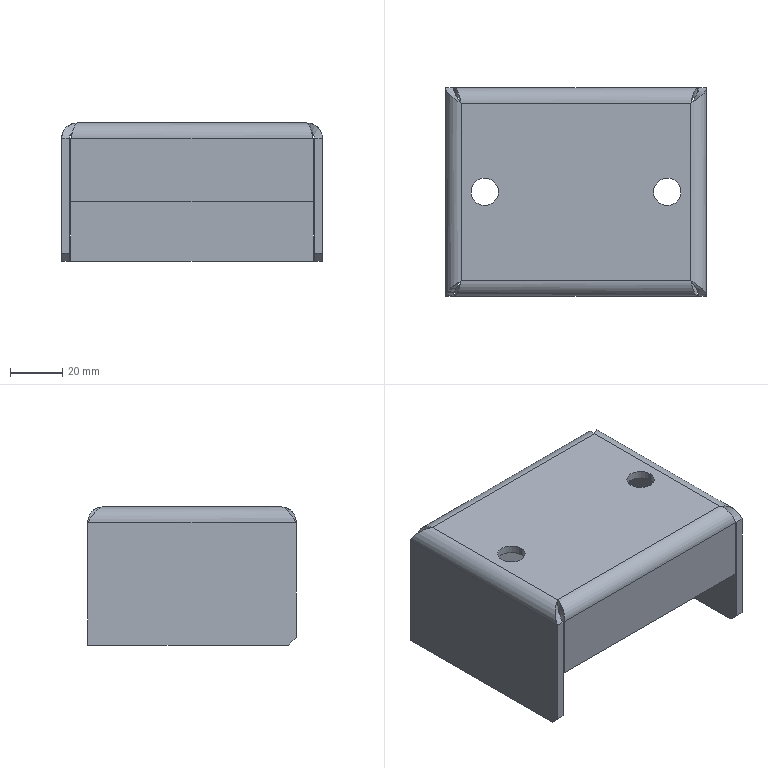Part | STEP file | SYL_0392D6J1SYL0380DJ10-1361819 | 1 solid | 44 faces | box 100 x 80 x 53 mm | volume 66751 mm3 | plane 24 | cylinder 12 | spline 8 | commonest cylinder face diameters 6 x4 10.5 x4 12 x4
STEP:
#1=CARTESIAN_POINT('',(29.75,0.,0.));
#2=VERTEX_POINT('',#1);
#3=CARTESIAN_POINT('',(29.75,0.,3.));
#4=VERTEX_POINT('',#3);
#5=CARTESIAN_POINT('',(29.75,0.,3.));
#6=DIRECTION('',(0.,0.,1.));
#7=VECTOR('',#6,1000.);
#8=LINE('',#5,#7);
#9=EDGE_CURVE('',#2,#4,#8,.T.);
#10=ORIENTED_EDGE('',*,*,#9,.F.);
#11=CARTESIAN_POINT('',(40.25,0.,0.));
#12=VERTEX_POINT('',#11);
#13=CARTESIAN_POINT('',(35.,0.,0.));
#14=DIRECTION('',(0.,0.,-1.));
#15=DIRECTION('',(-1.,0.,0.));
#16=AXIS2_PLACEMENT_3D('',#13,#14,#15);
#17=CIRCLE('',#16,5.25);
#18=EDGE_CURVE('',#2,#12,#17,.T.);
#19=ORIENTED_EDGE('',*,*,#18,.T.);
#20=CARTESIAN_POINT('',(40.25,0.,3.));
#21=VERTEX_POINT('',#20);
#22=CARTESIAN_POINT('',(40.25,0.,3.));
#23=DIRECTION('',(0.,0.,1.));
#24=VECTOR('',#23,1000.);
#25=LINE('',#22,#24);
#26=EDGE_CURVE('',#12,#21,#25,.T.);
#27=ORIENTED_EDGE('',*,*,#26,.T.);
#28=CARTESIAN_POINT('',(35.,0.,3.));
#29=DIRECTION('',(0.,0.,-1.));
#30=DIRECTION('',(-1.,0.,0.));
#31=AXIS2_PLACEMENT_3D('',#28,#29,#30);
#32=CIRCLE('',#31,5.25);
#33=EDGE_CURVE('',#4,#21,#32,.T.);
#34=ORIENTED_EDGE('',*,*,#33,.F.);
#35=EDGE_LOOP('',(#10,#19,#27,#34));
#36=FACE_OUTER_BOUND('',#35,.T.);
#37=CARTESIAN_POINT('',(35.,0.,3.));
#38=DIRECTION('',(0.,0.,1.));
#39=DIRECTION('',(1.,0.,0.));
#40=AXIS2_PLACEMENT_3D('',#37,#38,#39);
#41=CYLINDRICAL_SURFACE('',#40,5.25);
#42=ADVANCED_FACE('',(#36),#41,.F.);
#43=CARTESIAN_POINT('',(-40.25,0.,0.));
#44=VERTEX_POINT('',#43);
#45=CARTESIAN_POINT('',(-40.25,0.,3.));
#46=VERTEX_POINT('',#45);
#47=CARTESIAN_POINT('',(-40.25,0.,3.));
#48=DIRECTION('',(0.,0.,1.));
#49=VECTOR('',#48,1000.);
#50=LINE('',#47,#49);
#51=EDGE_CURVE('',#44,#46,#50,.T.);
#52=ORIENTED_EDGE('',*,*,#51,.F.);
#53=CARTESIAN_POINT('',(-29.75,0.,0.));
#54=VERTEX_POINT('',#53);
#55=CARTESIAN_POINT('',(-35.,0.,0.));
#56=DIRECTION('',(0.,0.,-1.));
#57=DIRECTION('',(-1.,0.,0.));
#58=AXIS2_PLACEMENT_3D('',#55,#56,#57);
#59=CIRCLE('',#58,5.25);
#60=EDGE_CURVE('',#44,#54,#59,.T.);
#61=ORIENTED_EDGE('',*,*,#60,.T.);
#62=CARTESIAN_POINT('',(-29.75,0.,3.));
#63=VERTEX_POINT('',#62);
#64=CARTESIAN_POINT('',(-29.75,0.,3.));
#65=DIRECTION('',(0.,0.,1.));
#66=VECTOR('',#65,1000.);
#67=LINE('',#64,#66);
#68=EDGE_CURVE('',#54,#63,#67,.T.);
#69=ORIENTED_EDGE('',*,*,#68,.T.);
#70=CARTESIAN_POINT('',(-35.,0.,3.));
#71=DIRECTION('',(0.,0.,-1.));
#72=DIRECTION('',(-1.,0.,0.));
#73=AXIS2_PLACEMENT_3D('',#70,#71,#72);
#74=CIRCLE('',#73,5.25);
#75=EDGE_CURVE('',#46,#63,#74,.T.);
#76=ORIENTED_EDGE('',*,*,#75,.F.);
#77=EDGE_LOOP('',(#52,#61,#69,#76));
#78=FACE_OUTER_BOUND('',#77,.T.);
#79=CARTESIAN_POINT('',(-35.,0.,3.));
#80=DIRECTION('',(0.,0.,1.));
#81=DIRECTION('',(1.,0.,0.));
#82=AXIS2_PLACEMENT_3D('',#79,#80,#81);
#83=CYLINDRICAL_SURFACE('',#82,5.25);
#84=ADVANCED_FACE('',(#78),#83,.F.);
#85=CARTESIAN_POINT('',(46.5,37.,-3.));
#86=VERTEX_POINT('',#85);
#87=CARTESIAN_POINT('',(46.5,40.,-3.));
#88=VERTEX_POINT('',#87);
#89=CARTESIAN_POINT('',(46.5,37.,-3.));
#90=CARTESIAN_POINT('',(46.5,40.,-3.));
#91=B_SPLINE_CURVE_WITH_KNOTS('',1,(#89,#90),.UNSPECIFIED.,.F.,.F.,(2,2),(0.,1.),.UNSPECIFIED.);
#92=EDGE_CURVE('',#86,#88,#91,.T.);
#93=ORIENTED_EDGE('',*,*,#92,.F.);
#94=CARTESIAN_POINT('',(46.5,37.,-50.));
#95=VERTEX_POINT('',#94);
#96=CARTESIAN_POINT('',(46.5,37.,3.));
#97=DIRECTION('',(0.,0.,1.));
#98=VECTOR('',#97,1000.);
#99=LINE('',#96,#98);
#100=EDGE_CURVE('',#95,#86,#99,.T.);
#101=ORIENTED_EDGE('',*,*,#100,.F.);
#102=CARTESIAN_POINT('',(46.5,40.,-50.));
#103=VERTEX_POINT('',#102);
#104=CARTESIAN_POINT('',(46.5,40.,-50.));
#105=DIRECTION('',(0.,1.,0.));
#106=VECTOR('',#105,1000.);
#107=LINE('',#104,#106);
#108=EDGE_CURVE('',#95,#103,#107,.T.);
#109=ORIENTED_EDGE('',*,*,#108,.T.);
#110=CARTESIAN_POINT('',(46.5,40.,-50.));
#111=DIRECTION('',(0.,0.,1.));
#112=VECTOR('',#111,1000.);
#113=LINE('',#110,#112);
#114=EDGE_CURVE('',#103,#88,#113,.T.);
#115=ORIENTED_EDGE('',*,*,#114,.T.);
#116=EDGE_LOOP('',(#93,#101,#109,#115));
#117=FACE_OUTER_BOUND('',#116,.T.);
#118=CARTESIAN_POINT('',(46.5,40.,-50.));
#119=DIRECTION('',(-1.,0.,0.));
#120=DIRECTION('',(0.,0.,1.));
#121=AXIS2_PLACEMENT_3D('',#118,#119,#120);
#122=PLANE('',#121);
#123=ADVANCED_FACE('',(#117),#122,.F.);
#124=ORIENTED_EDGE('',*,*,#108,.F.);
#125=CARTESIAN_POINT('',(-46.5,37.,-50.));
#126=VERTEX_POINT('',#125);
#127=CARTESIAN_POINT('',(44.,37.,-50.));
#128=DIRECTION('',(1.,0.,0.));
#129=VECTOR('',#128,1000.);
#130=LINE('',#127,#129);
#131=EDGE_CURVE('',#126,#95,#130,.T.);
#132=ORIENTED_EDGE('',*,*,#131,.F.);
#133=CARTESIAN_POINT('',(-46.5,40.,-50.));
#134=VERTEX_POINT('',#133);
#135=CARTESIAN_POINT('',(-46.5,40.,-50.));
#136=DIRECTION('',(0.,1.,0.));
#137=VECTOR('',#136,1000.);
#138=LINE('',#135,#137);
#139=EDGE_CURVE('',#126,#134,#138,.T.);
#140=ORIENTED_EDGE('',*,*,#139,.T.);
#141=CARTESIAN_POINT('',(-46.5,40.,-50.));
#142=DIRECTION('',(1.,0.,0.));
#143=VECTOR('',#142,1000.);
#144=LINE('',#141,#143);
#145=EDGE_CURVE('',#134,#103,#144,.T.);
#146=ORIENTED_EDGE('',*,*,#145,.T.);
#147=EDGE_LOOP('',(#124,#132,#140,#146));
#148=FACE_OUTER_BOUND('',#147,.T.);
#149=CARTESIAN_POINT('',(-46.5,40.,-50.));
#150=DIRECTION('',(0.,0.,1.));
#151=DIRECTION('',(1.,0.,0.));
#152=AXIS2_PLACEMENT_3D('',#149,#150,#151);
#153=PLANE('',#152);
#154=ADVANCED_FACE('',(#148),#153,.F.);
#155=ORIENTED_EDGE('',*,*,#139,.F.);
#156=CARTESIAN_POINT('',(-46.5,37.,-3.));
#157=VERTEX_POINT('',#156);
#158=CARTESIAN_POINT('',(-46.5,37.,3.));
#159=DIRECTION('',(0.,0.,1.));
#160=VECTOR('',#159,1000.);
#161=LINE('',#158,#160);
#162=EDGE_CURVE('',#126,#157,#161,.T.);
#163=ORIENTED_EDGE('',*,*,#162,.T.);
#164=CARTESIAN_POINT('',(-46.5,40.,-3.));
#165=VERTEX_POINT('',#164);
#166=CARTESIAN_POINT('',(-46.5,37.,-3.));
#167=CARTESIAN_POINT('',(-46.5,38.,-3.));
#168=CARTESIAN_POINT('',(-46.5,39.,-3.));
#169=CARTESIAN_POINT('',(-46.5,40.,-3.));
#170=B_SPLINE_CURVE_WITH_KNOTS('',3,(#166,#167,#168,#169),.UNSPECIFIED.,.F.,.F.,(4,4),(0.,1.),.UNSPECIFIED.);
#171=EDGE_CURVE('',#157,#165,#170,.T.);
#172=ORIENTED_EDGE('',*,*,#171,.T.);
#173=CARTESIAN_POINT('',(-46.5,40.,-50.));
#174=DIRECTION('',(0.,0.,1.));
#175=VECTOR('',#174,1000.);
#176=LINE('',#173,#175);
#177=EDGE_CURVE('',#134,#165,#176,.T.);
#178=ORIENTED_EDGE('',*,*,#177,.F.);
#179=EDGE_LOOP('',(#155,#163,#172,#178));
#180=FACE_OUTER_BOUND('',#179,.T.);
#181=CARTESIAN_POINT('',(-46.5,40.,-50.));
#182=DIRECTION('',(-1.,0.,0.));
#183=DIRECTION('',(0.,0.,1.));
#184=AXIS2_PLACEMENT_3D('',#181,#182,#183);
#185=PLANE('',#184);
#186=ADVANCED_FACE('',(#180),#185,.T.);
#187=ORIENTED_EDGE('',*,*,#171,.F.);
#188=CARTESIAN_POINT('',(-44.,34.,0.));
#189=VERTEX_POINT('',#188);
#190=CARTESIAN_POINT('',(-46.5,37.,-3.));
#191=CARTESIAN_POINT('',(-46.292,37.,-2.607));
#192=CARTESIAN_POINT('',(-46.083,36.922,-2.215));
#193=CARTESIAN_POINT('',(-45.667,36.621,-1.489));
#194=CARTESIAN_POINT('',(-45.458,36.399,-1.156));
#195=CARTESIAN_POINT('',(-45.042,35.844,-0.601));
#196=CARTESIAN_POINT('',(-44.833,35.511,-0.3786));
#197=CARTESIAN_POINT('',(-44.417,34.785,-0.07808));
#198=CARTESIAN_POINT('',(-44.208,34.393,0.));
#199=CARTESIAN_POINT('',(-44.,34.,0.));
#200=B_SPLINE_CURVE_WITH_KNOTS('',3,(#190,#191,#192,#193,#194,#195,#196,#197,#198,#199),.UNSPECIFIED.,.F.,.F.,(4,2,2,2,4),(0.,0.25,0.5,0.75,1.),.UNSPECIFIED.);
#201=EDGE_CURVE('',#157,#189,#200,.T.);
#202=ORIENTED_EDGE('',*,*,#201,.T.);
#203=CARTESIAN_POINT('',(-44.,34.,3.));
#204=VERTEX_POINT('',#203);
#205=CARTESIAN_POINT('',(-44.,34.,0.));
#206=CARTESIAN_POINT('',(-44.,34.,3.));
#207=B_SPLINE_CURVE_WITH_KNOTS('',1,(#205,#206),.UNSPECIFIED.,.F.,.F.,(2,2),(0.,1.),.UNSPECIFIED.);
#208=EDGE_CURVE('',#189,#204,#207,.T.);
#209=ORIENTED_EDGE('',*,*,#208,.T.);
#210=CARTESIAN_POINT('',(-46.5,40.,-3.));
#211=CARTESIAN_POINT('',(-46.292,40.,-2.215));
#212=CARTESIAN_POINT('',(-46.083,39.844,-1.43));
#213=CARTESIAN_POINT('',(-45.667,39.243,0.02171));
#214=CARTESIAN_POINT('',(-45.458,38.798,0.6873));
#215=CARTESIAN_POINT('',(-45.042,37.687,1.798));
#216=CARTESIAN_POINT('',(-44.833,37.022,2.243));
#217=CARTESIAN_POINT('',(-44.417,35.57,2.844));
#218=CARTESIAN_POINT('',(-44.208,34.785,3.));
#219=CARTESIAN_POINT('',(-44.,34.,3.));
#220=B_SPLINE_CURVE_WITH_KNOTS('',3,(#210,#211,#212,#213,#214,#215,#216,#217,#218,#219),.UNSPECIFIED.,.F.,.F.,(4,2,2,2,4),(0.,0.25,0.5,0.75,1.),.UNSPECIFIED.);
#221=EDGE_CURVE('',#165,#204,#220,.T.);
#222=ORIENTED_EDGE('',*,*,#221,.F.);
#223=EDGE_LOOP('',(#187,#202,#209,#222));
#224=FACE_OUTER_BOUND('',#223,.T.);
#225=CARTESIAN_POINT('',(-46.5,40.,-3.));
#226=CARTESIAN_POINT('',(-46.292,40.,-2.214));
#227=CARTESIAN_POINT('',(-46.083,39.844,-1.43));
#228=CARTESIAN_POINT('',(-45.667,39.243,0.02171));
#229=CARTESIAN_POINT('',(-45.458,38.798,0.6873));
#230=CARTESIAN_POINT('',(-45.042,37.687,1.798));
#231=CARTESIAN_POINT('',(-44.833,37.022,2.243));
#232=CARTESIAN_POINT('',(-44.417,35.57,2.844));
#233=CARTESIAN_POINT('',(-44.208,34.786,3.));
#234=CARTESIAN_POINT('',(-44.,34.,3.));
#235=CARTESIAN_POINT('',(-46.5,37.,-3.));
#236=CARTESIAN_POINT('',(-46.292,37.,-2.607));
#237=CARTESIAN_POINT('',(-46.083,36.922,-2.215));
#238=CARTESIAN_POINT('',(-45.667,36.621,-1.489));
#239=CARTESIAN_POINT('',(-45.458,36.399,-1.156));
#240=CARTESIAN_POINT('',(-45.042,35.844,-0.601));
#241=CARTESIAN_POINT('',(-44.833,35.511,-0.3786));
#242=CARTESIAN_POINT('',(-44.417,34.785,-0.07808));
#243=CARTESIAN_POINT('',(-44.208,34.393,0.));
#244=CARTESIAN_POINT('',(-44.,34.,0.));
#245=B_SPLINE_SURFACE_WITH_KNOTS('',1,3,((#225,#226,#227,#228,#229,#230,#231,#232,#233,#234),(#235,#236,#237,#238,#239,#240,#241,#242,#243,#244)),.UNSPECIFIED.,.F.,.F.,.F.,(2,2),(4,2,2,2,4),(0.,1.),(0.,0.25,0.5,0.75,1.),.UNSPECIFIED.);
#246=ADVANCED_FACE('',(#224),#245,.T.);
#247=ORIENTED_EDGE('',*,*,#208,.F.);
#248=CARTESIAN_POINT('',(-47.,40.,-3.));
#249=VERTEX_POINT('',#248);
#250=CARTESIAN_POINT('',(-44.,34.,0.));
#251=CARTESIAN_POINT('',(-44.393,34.5,0.));
#252=CARTESIAN_POINT('',(-44.785,35.,-0.07808));
#253=CARTESIAN_POINT('',(-45.511,36.,-0.3786));
#254=CARTESIAN_POINT('',(-45.844,36.5,-0.601));
#255=CARTESIAN_POINT('',(-46.399,37.5,-1.156));
#256=CARTESIAN_POINT('',(-46.621,38.,-1.489));
#257=CARTESIAN_POINT('',(-46.922,39.,-2.215));
#258=CARTESIAN_POINT('',(-47.,39.5,-2.607));
#259=CARTESIAN_POINT('',(-47.,40.,-3.));
#260=B_SPLINE_CURVE_WITH_KNOTS('',3,(#250,#251,#252,#253,#254,#255,#256,#257,#258,#259),.UNSPECIFIED.,.F.,.F.,(4,2,2,2,4),(0.,0.25,0.5,0.75,1.),.UNSPECIFIED.);
#261=EDGE_CURVE('',#189,#249,#260,.T.);
#262=ORIENTED_EDGE('',*,*,#261,.T.);
#263=CARTESIAN_POINT('',(-50.,40.,-3.));
#264=VERTEX_POINT('',#263);
#265=CARTESIAN_POINT('',(-47.,40.,-3.));
#266=CARTESIAN_POINT('',(-50.,40.,-3.));
#267=B_SPLINE_CURVE_WITH_KNOTS('',1,(#265,#266),.UNSPECIFIED.,.F.,.F.,(2,2),(0.,1.),.UNSPECIFIED.);
#268=EDGE_CURVE('',#249,#264,#267,.T.);
#269=ORIENTED_EDGE('',*,*,#268,.T.);
#270=CARTESIAN_POINT('',(-44.,34.,3.));
#271=CARTESIAN_POINT('',(-44.785,34.5,3.));
#272=CARTESIAN_POINT('',(-45.57,35.,2.844));
#273=CARTESIAN_POINT('',(-47.022,36.,2.243));
#274=CARTESIAN_POINT('',(-47.687,36.5,1.798));
#275=CARTESIAN_POINT('',(-48.798,37.5,0.6873));
#276=CARTESIAN_POINT('',(-49.243,38.,0.02171));
#277=CARTESIAN_POINT('',(-49.844,39.,-1.43));
#278=CARTESIAN_POINT('',(-50.,39.5,-2.215));
#279=CARTESIAN_POINT('',(-50.,40.,-3.));
#280=B_SPLINE_CURVE_WITH_KNOTS('',3,(#270,#271,#272,#273,#274,#275,#276,#277,#278,#279),.UNSPECIFIED.,.F.,.F.,(4,2,2,2,4),(0.,0.25,0.5,0.75,1.),.UNSPECIFIED.);
#281=EDGE_CURVE('',#204,#264,#280,.T.);
#282=ORIENTED_EDGE('',*,*,#281,.F.);
#283=EDGE_LOOP('',(#247,#262,#269,#282));
#284=FACE_OUTER_BOUND('',#283,.T.);
#285=CARTESIAN_POINT('',(-44.,34.,3.));
#286=CARTESIAN_POINT('',(-44.785,34.5,3.));
#287=CARTESIAN_POINT('',(-45.57,35.,2.844));
#288=CARTESIAN_POINT('',(-47.022,36.,2.243));
#289=CARTESIAN_POINT('',(-47.687,36.5,1.798));
#290=CARTESIAN_POINT('',(-48.798,37.5,0.6873));
#291=CARTESIAN_POINT('',(-49.243,38.,0.02171));
#292=CARTESIAN_POINT('',(-49.844,39.,-1.43));
#293=CARTESIAN_POINT('',(-50.,39.5,-2.215));
#294=CARTESIAN_POINT('',(-50.,40.,-3.));
#295=CARTESIAN_POINT('',(-44.,34.,0.));
#296=CARTESIAN_POINT('',(-44.393,34.5,0.));
#297=CARTESIAN_POINT('',(-44.785,35.,-0.07808));
#298=CARTESIAN_POINT('',(-45.511,36.,-0.3786));
#299=CARTESIAN_POINT('',(-45.844,36.5,-0.601));
#300=CARTESIAN_POINT('',(-46.399,37.5,-1.156));
#301=CARTESIAN_POINT('',(-46.621,38.,-1.489));
#302=CARTESIAN_POINT('',(-46.922,39.,-2.215));
#303=CARTESIAN_POINT('',(-47.,39.5,-2.607));
#304=CARTESIAN_POINT('',(-47.,40.,-3.));
#305=B_SPLINE_SURFACE_WITH_KNOTS('',1,3,((#285,#286,#287,#288,#289,#290,#291,#292,#293,#294),(#295,#296,#297,#298,#299,#300,#301,#302,#303,#304)),.UNSPECIFIED.,.F.,.F.,.F.,(2,2),(4,2,2,2,4),(0.,1.),(0.,0.25,0.5,0.75,1.),.UNSPECIFIED.);
#306=ADVANCED_FACE('',(#284),#305,.T.);
#307=ORIENTED_EDGE('',*,*,#268,.F.);
#308=CARTESIAN_POINT('',(-47.,40.,-50.));
#309=VERTEX_POINT('',#308);
#310=CARTESIAN_POINT('',(-47.,40.,3.));
#311=DIRECTION('',(0.,0.,1.));
#312=VECTOR('',#311,1000.);
#313=LINE('',#310,#312);
#314=EDGE_CURVE('',#309,#249,#313,.T.);
#315=ORIENTED_EDGE('',*,*,#314,.F.);
#316=CARTESIAN_POINT('',(-50.,40.,-50.));
#317=VERTEX_POINT('',#316);
#318=CARTESIAN_POINT('',(-50.,40.,-50.));
#319=DIRECTION('',(-1.,0.,0.));
#320=VECTOR('',#319,1000.);
#321=LINE('',#318,#320);
#322=EDGE_CURVE('',#309,#317,#321,.T.);
#323=ORIENTED_EDGE('',*,*,#322,.T.);
#324=CARTESIAN_POINT('',(-50.,40.,-50.));
#325=DIRECTION('',(0.,0.,1.));
#326=VECTOR('',#325,1000.);
#327=LINE('',#324,#326);
#328=EDGE_CURVE('',#317,#264,#327,.T.);
#329=ORIENTED_EDGE('',*,*,#328,.T.);
#330=EDGE_LOOP('',(#307,#315,#323,#329));
#331=FACE_OUTER_BOUND('',#330,.T.);
#332=CARTESIAN_POINT('',(-50.,40.,-50.));
#333=DIRECTION('',(0.,-1.,0.));
#334=DIRECTION('',(0.,0.,1.));
#335=AXIS2_PLACEMENT_3D('',#332,#333,#334);
#336=PLANE('',#335);
#337=ADVANCED_FACE('',(#331),#336,.F.);
#338=ORIENTED_EDGE('',*,*,#322,.F.);
#339=CARTESIAN_POINT('',(-47.,-37.,-50.));
#340=VERTEX_POINT('',#339);
#341=CARTESIAN_POINT('',(-47.,40.,-50.));
#342=DIRECTION('',(0.,1.,0.));
#343=VECTOR('',#342,1000.);
#344=LINE('',#341,#343);
#345=EDGE_CURVE('',#340,#309,#344,.T.);
#346=ORIENTED_EDGE('',*,*,#345,.F.);
#347=CARTESIAN_POINT('',(-50.,-37.,-50.));
#348=VERTEX_POINT('',#347);
#349=CARTESIAN_POINT('',(-50.,-37.,-50.));
#350=DIRECTION('',(-1.,0.,0.));
#351=VECTOR('',#350,1000.);
#352=LINE('',#349,#351);
#353=EDGE_CURVE('',#340,#348,#352,.T.);
#354=ORIENTED_EDGE('',*,*,#353,.T.);
#355=CARTESIAN_POINT('',(-50.,-37.,-50.));
#356=DIRECTION('',(0.,1.,0.));
#357=VECTOR('',#356,1000.);
#358=LINE('',#355,#357);
#359=EDGE_CURVE('',#348,#317,#358,.T.);
#360=ORIENTED_EDGE('',*,*,#359,.T.);
#361=EDGE_LOOP('',(#338,#346,#354,#360));
#362=FACE_OUTER_BOUND('',#361,.T.);
#363=CARTESIAN_POINT('',(-50.,-37.,-50.));
#364=DIRECTION('',(0.,0.,1.));
#365=DIRECTION('',(0.,1.,0.));
#366=AXIS2_PLACEMENT_3D('',#363,#364,#365);
#367=PLANE('',#366);
#368=ADVANCED_FACE('',(#362),#367,.F.);
#369=ORIENTED_EDGE('',*,*,#353,.F.);
#370=CARTESIAN_POINT('',(-47.,-40.,-47.));
#371=VERTEX_POINT('',#370);
#372=CARTESIAN_POINT('',(-47.,-37.,-50.));
#373=DIRECTION('',(0.,-0.7071,0.7071));
#374=VECTOR('',#373,1000.);
#375=LINE('',#372,#374);
#376=EDGE_CURVE('',#340,#371,#375,.T.);
#377=ORIENTED_EDGE('',*,*,#376,.T.);
#378=CARTESIAN_POINT('',(-50.,-40.,-47.));
#379=VERTEX_POINT('',#378);
#380=CARTESIAN_POINT('',(-50.,-40.,-47.));
#381=DIRECTION('',(-1.,0.,0.));
#382=VECTOR('',#381,1000.);
#383=LINE('',#380,#382);
#384=EDGE_CURVE('',#371,#379,#383,.T.);
#385=ORIENTED_EDGE('',*,*,#384,.T.);
#386=CARTESIAN_POINT('',(-50.,-37.,-50.));
#387=DIRECTION('',(0.,-0.7071,0.7071));
#388=VECTOR('',#387,1000.);
#389=LINE('',#386,#388);
#390=EDGE_CURVE('',#348,#379,#389,.T.);
#391=ORIENTED_EDGE('',*,*,#390,.F.);
#392=EDGE_LOOP('',(#369,#377,#385,#391));
#393=FACE_OUTER_BOUND('',#392,.T.);
#394=CARTESIAN_POINT('',(-50.,-37.,-50.));
#395=DIRECTION('',(0.,-0.7071,-0.7071));
#396=DIRECTION('',(0.,-0.7071,0.7071));
#397=AXIS2_PLACEMENT_3D('',#394,#395,#396);
#398=PLANE('',#397);
#399=ADVANCED_FACE('',(#393),#398,.T.);
#400=ORIENTED_EDGE('',*,*,#384,.F.);
#401=CARTESIAN_POINT('',(-47.,-40.,-3.));
#402=VERTEX_POINT('',#401);
#403=CARTESIAN_POINT('',(-47.,-40.,3.));
#404=DIRECTION('',(0.,0.,1.));
#405=VECTOR('',#404,1000.);
#406=LINE('',#403,#405);
#407=EDGE_CURVE('',#371,#402,#406,.T.);
#408=ORIENTED_EDGE('',*,*,#407,.T.);
#409=CARTESIAN_POINT('',(-50.,-40.,-3.));
#410=VERTEX_POINT('',#409);
#411=CARTESIAN_POINT('',(-47.,-40.,-3.));
#412=CARTESIAN_POINT('',(-48.,-40.,-3.));
#413=CARTESIAN_POINT('',(-49.,-40.,-3.));
#414=CARTESIAN_POINT('',(-50.,-40.,-3.));
#415=B_SPLINE_CURVE_WITH_KNOTS('',3,(#411,#412,#413,#414),.UNSPECIFIED.,.F.,.F.,(4,4),(0.,1.),.UNSPECIFIED.);
#416=EDGE_CURVE('',#402,#410,#415,.T.);
#417=ORIENTED_EDGE('',*,*,#416,.T.);
#418=CARTESIAN_POINT('',(-50.,-40.,-47.));
#419=DIRECTION('',(0.,0.,1.));
#420=VECTOR('',#419,1000.);
#421=LINE('',#418,#420);
#422=EDGE_CURVE('',#379,#410,#421,.T.);
#423=ORIENTED_EDGE('',*,*,#422,.F.);
#424=EDGE_LOOP('',(#400,#408,#417,#423));
#425=FACE_OUTER_BOUND('',#424,.T.);
#426=CARTESIAN_POINT('',(-50.,-40.,-47.));
#427=DIRECTION('',(0.,-1.,0.));
#428=DIRECTION('',(0.,0.,1.));
#429=AXIS2_PLACEMENT_3D('',#426,#427,#428);
#430=PLANE('',#429);
#431=ADVANCED_FACE('',(#425),#430,.T.);
#432=ORIENTED_EDGE('',*,*,#416,.F.);
#433=CARTESIAN_POINT('',(-44.,-34.,0.));
#434=VERTEX_POINT('',#433);
#435=CARTESIAN_POINT('',(-47.,-40.,-3.));
#436=CARTESIAN_POINT('',(-47.,-39.5,-2.607));
#437=CARTESIAN_POINT('',(-46.922,-39.,-2.215));
#438=CARTESIAN_POINT('',(-46.621,-38.,-1.489));
#439=CARTESIAN_POINT('',(-46.399,-37.5,-1.156));
#440=CARTESIAN_POINT('',(-45.844,-36.5,-0.601));
#441=CARTESIAN_POINT('',(-45.511,-36.,-0.3786));
#442=CARTESIAN_POINT('',(-44.785,-35.,-0.07808));
#443=CARTESIAN_POINT('',(-44.393,-34.5,0.));
#444=CARTESIAN_POINT('',(-44.,-34.,0.));
#445=B_SPLINE_CURVE_WITH_KNOTS('',3,(#435,#436,#437,#438,#439,#440,#441,#442,#443,#444),.UNSPECIFIED.,.F.,.F.,(4,2,2,2,4),(0.,0.25,0.5,0.75,1.),.UNSPECIFIED.);
#446=EDGE_CURVE('',#402,#434,#445,.T.);
#447=ORIENTED_EDGE('',*,*,#446,.T.);
#448=CARTESIAN_POINT('',(-44.,-34.,3.));
#449=VERTEX_POINT('',#448);
#450=CARTESIAN_POINT('',(-44.,-34.,0.));
#451=CARTESIAN_POINT('',(-44.,-34.,3.));
#452=B_SPLINE_CURVE_WITH_KNOTS('',1,(#450,#451),.UNSPECIFIED.,.F.,.F.,(2,2),(0.,1.),.UNSPECIFIED.);
#453=EDGE_CURVE('',#434,#449,#452,.T.);
#454=ORIENTED_EDGE('',*,*,#453,.T.);
#455=CARTESIAN_POINT('',(-50.,-40.,-3.));
#456=CARTESIAN_POINT('',(-50.,-39.5,-2.215));
#457=CARTESIAN_POINT('',(-49.844,-39.,-1.43));
#458=CARTESIAN_POINT('',(-49.243,-38.,0.02171));
#459=CARTESIAN_POINT('',(-48.798,-37.5,0.6873));
#460=CARTESIAN_POINT('',(-47.687,-36.5,1.798));
#461=CARTESIAN_POINT('',(-47.022,-36.,2.243));
#462=CARTESIAN_POINT('',(-45.57,-35.,2.844));
#463=CARTESIAN_POINT('',(-44.785,-34.5,3.));
#464=CARTESIAN_POINT('',(-44.,-34.,3.));
#465=B_SPLINE_CURVE_WITH_KNOTS('',3,(#455,#456,#457,#458,#459,#460,#461,#462,#463,#464),.UNSPECIFIED.,.F.,.F.,(4,2,2,2,4),(0.,0.25,0.5,0.75,1.),.UNSPECIFIED.);
#466=EDGE_CURVE('',#410,#449,#465,.T.);
#467=ORIENTED_EDGE('',*,*,#466,.F.);
#468=EDGE_LOOP('',(#432,#447,#454,#467));
#469=FACE_OUTER_BOUND('',#468,.T.);
#470=CARTESIAN_POINT('',(-50.,-40.,-3.));
#471=CARTESIAN_POINT('',(-50.,-39.5,-2.215));
#472=CARTESIAN_POINT('',(-49.844,-39.,-1.43));
#473=CARTESIAN_POINT('',(-49.243,-38.,0.02171));
#474=CARTESIAN_POINT('',(-48.798,-37.5,0.6873));
#475=CARTESIAN_POINT('',(-47.687,-36.5,1.798));
#476=CARTESIAN_POINT('',(-47.022,-36.,2.243));
#477=CARTESIAN_POINT('',(-45.57,-35.,2.844));
#478=CARTESIAN_POINT('',(-44.785,-34.5,3.));
#479=CARTESIAN_POINT('',(-44.,-34.,3.));
#480=CARTESIAN_POINT('',(-47.,-40.,-3.));
#481=CARTESIAN_POINT('',(-47.,-39.5,-2.607));
#482=CARTESIAN_POINT('',(-46.922,-39.,-2.215));
#483=CARTESIAN_POINT('',(-46.621,-38.,-1.489));
#484=CARTESIAN_POINT('',(-46.399,-37.5,-1.156));
#485=CARTESIAN_POINT('',(-45.844,-36.5,-0.601));
#486=CARTESIAN_POINT('',(-45.511,-36.,-0.3786));
#487=CARTESIAN_POINT('',(-44.785,-35.,-0.07808));
#488=CARTESIAN_POINT('',(-44.393,-34.5,0.));
#489=CARTESIAN_POINT('',(-44.,-34.,0.));
#490=B_SPLINE_SURFACE_WITH_KNOTS('',1,3,((#470,#471,#472,#473,#474,#475,#476,#477,#478,#479),(#480,#481,#482,#483,#484,#485,#486,#487,#488,#489)),.UNSPECIFIED.,.F.,.F.,.F.,(2,2),(4,2,2,2,4),(0.,1.),(0.,0.25,0.5,0.75,1.),.UNSPECIFIED.);
#491=ADVANCED_FACE('',(#469),#490,.T.);
#492=ORIENTED_EDGE('',*,*,#453,.F.);
#493=CARTESIAN_POINT('',(-46.5,-37.,-3.));
#494=VERTEX_POINT('',#493);
#495=CARTESIAN_POINT('',(-44.,-34.,0.));
#496=CARTESIAN_POINT('',(-44.208,-34.393,0.));
#497=CARTESIAN_POINT('',(-44.417,-34.785,-0.07808));
#498=CARTESIAN_POINT('',(-44.833,-35.511,-0.3786));
#499=CARTESIAN_POINT('',(-45.042,-35.844,-0.601));
#500=CARTESIAN_POINT('',(-45.458,-36.399,-1.156));
#501=CARTESIAN_POINT('',(-45.667,-36.621,-1.489));
#502=CARTESIAN_POINT('',(-46.083,-36.922,-2.215));
#503=CARTESIAN_POINT('',(-46.292,-37.,-2.607));
#504=CARTESIAN_POINT('',(-46.5,-37.,-3.));
#505=B_SPLINE_CURVE_WITH_KNOTS('',3,(#495,#496,#497,#498,#499,#500,#501,#502,#503,#504),.UNSPECIFIED.,.F.,.F.,(4,2,2,2,4),(0.,0.25,0.5,0.75,1.),.UNSPECIFIED.);
#506=EDGE_CURVE('',#434,#494,#505,.T.);
#507=ORIENTED_EDGE('',*,*,#506,.T.);
#508=CARTESIAN_POINT('',(-46.5,-40.,-3.));
#509=VERTEX_POINT('',#508);
#510=CARTESIAN_POINT('',(-46.5,-37.,-3.));
#511=CARTESIAN_POINT('',(-46.5,-40.,-3.));
#512=B_SPLINE_CURVE_WITH_KNOTS('',1,(#510,#511),.UNSPECIFIED.,.F.,.F.,(2,2),(0.,1.),.UNSPECIFIED.);
#513=EDGE_CURVE('',#494,#509,#512,.T.);
#514=ORIENTED_EDGE('',*,*,#513,.T.);
#515=CARTESIAN_POINT('',(-44.,-34.,3.));
#516=CARTESIAN_POINT('',(-44.208,-34.785,3.));
#517=CARTESIAN_POINT('',(-44.417,-35.57,2.844));
#518=CARTESIAN_POINT('',(-44.833,-37.022,2.243));
#519=CARTESIAN_POINT('',(-45.042,-37.687,1.798));
#520=CARTESIAN_POINT('',(-45.458,-38.798,0.6873));
#521=CARTESIAN_POINT('',(-45.667,-39.243,0.02171));
#522=CARTESIAN_POINT('',(-46.083,-39.844,-1.43));
#523=CARTESIAN_POINT('',(-46.292,-40.,-2.215));
#524=CARTESIAN_POINT('',(-46.5,-40.,-3.));
#525=B_SPLINE_CURVE_WITH_KNOTS('',3,(#515,#516,#517,#518,#519,#520,#521,#522,#523,#524),.UNSPECIFIED.,.F.,.F.,(4,2,2,2,4),(0.,0.25,0.5,0.75,1.),.UNSPECIFIED.);
#526=EDGE_CURVE('',#449,#509,#525,.T.);
#527=ORIENTED_EDGE('',*,*,#526,.F.);
#528=EDGE_LOOP('',(#492,#507,#514,#527));
#529=FACE_OUTER_BOUND('',#528,.T.);
#530=CARTESIAN_POINT('',(-44.,-34.,3.));
#531=CARTESIAN_POINT('',(-44.208,-34.786,3.));
#532=CARTESIAN_POINT('',(-44.417,-35.57,2.844));
#533=CARTESIAN_POINT('',(-44.833,-37.022,2.243));
#534=CARTESIAN_POINT('',(-45.042,-37.687,1.798));
#535=CARTESIAN_POINT('',(-45.458,-38.798,0.6873));
#536=CARTESIAN_POINT('',(-45.667,-39.243,0.02171));
#537=CARTESIAN_POINT('',(-46.083,-39.844,-1.43));
#538=CARTESIAN_POINT('',(-46.292,-40.,-2.214));
#539=CARTESIAN_POINT('',(-46.5,-40.,-3.));
#540=CARTESIAN_POINT('',(-44.,-34.,0.));
#541=CARTESIAN_POINT('',(-44.208,-34.393,0.));
#542=CARTESIAN_POINT('',(-44.417,-34.785,-0.07808));
#543=CARTESIAN_POINT('',(-44.833,-35.511,-0.3786));
#544=CARTESIAN_POINT('',(-45.042,-35.844,-0.601));
#545=CARTESIAN_POINT('',(-45.458,-36.399,-1.156));
#546=CARTESIAN_POINT('',(-45.667,-36.621,-1.489));
#547=CARTESIAN_POINT('',(-46.083,-36.922,-2.215));
#548=CARTESIAN_POINT('',(-46.292,-37.,-2.607));
#549=CARTESIAN_POINT('',(-46.5,-37.,-3.));
#550=B_SPLINE_SURFACE_WITH_KNOTS('',1,3,((#530,#531,#532,#533,#534,#535,#536,#537,#538,#539),(#540,#541,#542,#543,#544,#545,#546,#547,#548,#549)),.UNSPECIFIED.,.F.,.F.,.F.,(2,2),(4,2,2,2,4),(0.,1.),(0.,0.25,0.5,0.75,1.),.UNSPECIFIED.);
#551=ADVANCED_FACE('',(#529),#550,.T.);
#552=ORIENTED_EDGE('',*,*,#513,.F.);
#553=CARTESIAN_POINT('',(-46.5,-37.,-27.));
#554=VERTEX_POINT('',#553);
#555=CARTESIAN_POINT('',(-46.5,-37.,3.));
#556=DIRECTION('',(0.,0.,1.));
#557=VECTOR('',#556,1000.);
#558=LINE('',#555,#557);
#559=EDGE_CURVE('',#554,#494,#558,.T.);
#560=ORIENTED_EDGE('',*,*,#559,.F.);
#561=CARTESIAN_POINT('',(-46.5,-40.,-27.));
#562=VERTEX_POINT('',#561);
#563=CARTESIAN_POINT('',(-46.5,-40.,-27.));
#564=DIRECTION('',(0.,-1.,0.));
#565=VECTOR('',#564,1000.);
#566=LINE('',#563,#565);
#567=EDGE_CURVE('',#554,#562,#566,.T.);
#568=ORIENTED_EDGE('',*,*,#567,.T.);
#569=CARTESIAN_POINT('',(-46.5,-40.,-27.));
#570=DIRECTION('',(0.,0.,1.));
#571=VECTOR('',#570,1000.);
#572=LINE('',#569,#571);
#573=EDGE_CURVE('',#562,#509,#572,.T.);
#574=ORIENTED_EDGE('',*,*,#573,.T.);
#575=EDGE_LOOP('',(#552,#560,#568,#574));
#576=FACE_OUTER_BOUND('',#575,.T.);
#577=CARTESIAN_POINT('',(-46.5,-40.,-27.));
#578=DIRECTION('',(1.,0.,0.));
#579=DIRECTION('',(0.,0.,1.));
#580=AXIS2_PLACEMENT_3D('',#577,#578,#579);
#581=PLANE('',#580);
#582=ADVANCED_FACE('',(#576),#581,.F.);
#583=ORIENTED_EDGE('',*,*,#567,.F.);
#584=CARTESIAN_POINT('',(46.5,-37.,-27.));
#585=VERTEX_POINT('',#584);
#586=CARTESIAN_POINT('',(-44.,-37.,-27.));
#587=DIRECTION('',(-1.,0.,0.));
#588=VECTOR('',#587,1000.);
#589=LINE('',#586,#588);
#590=EDGE_CURVE('',#585,#554,#589,.T.);
#591=ORIENTED_EDGE('',*,*,#590,.F.);
#592=CARTESIAN_POINT('',(46.5,-40.,-27.));
#593=VERTEX_POINT('',#592);
#594=CARTESIAN_POINT('',(46.5,-40.,-27.));
#595=DIRECTION('',(0.,-1.,0.));
#596=VECTOR('',#595,1000.);
#597=LINE('',#594,#596);
#598=EDGE_CURVE('',#585,#593,#597,.T.);
#599=ORIENTED_EDGE('',*,*,#598,.T.);
#600=CARTESIAN_POINT('',(46.5,-40.,-27.));
#601=DIRECTION('',(-1.,0.,0.));
#602=VECTOR('',#601,1000.);
#603=LINE('',#600,#602);
#604=EDGE_CURVE('',#593,#562,#603,.T.);
#605=ORIENTED_EDGE('',*,*,#604,.T.);
#606=EDGE_LOOP('',(#583,#591,#599,#605));
#607=FACE_OUTER_BOUND('',#606,.T.);
#608=CARTESIAN_POINT('',(46.5,-40.,-27.));
#609=DIRECTION('',(0.,0.,1.));
#610=DIRECTION('',(-1.,0.,0.));
#611=AXIS2_PLACEMENT_3D('',#608,#609,#610);
#612=PLANE('',#611);
#613=ADVANCED_FACE('',(#607),#612,.F.);
#614=ORIENTED_EDGE('',*,*,#598,.F.);
#615=CARTESIAN_POINT('',(46.5,-37.,-3.));
#616=VERTEX_POINT('',#615);
#617=CARTESIAN_POINT('',(46.5,-37.,3.));
#618=DIRECTION('',(0.,0.,1.));
#619=VECTOR('',#618,1000.);
#620=LINE('',#617,#619);
#621=EDGE_CURVE('',#585,#616,#620,.T.);
#622=ORIENTED_EDGE('',*,*,#621,.T.);
#623=CARTESIAN_POINT('',(46.5,-40.,-3.));
#624=VERTEX_POINT('',#623);
#625=CARTESIAN_POINT('',(46.5,-37.,-3.));
#626=CARTESIAN_POINT('',(46.5,-38.,-3.));
#627=CARTESIAN_POINT('',(46.5,-39.,-3.));
#628=CARTESIAN_POINT('',(46.5,-40.,-3.));
#629=B_SPLINE_CURVE_WITH_KNOTS('',3,(#625,#626,#627,#628),.UNSPECIFIED.,.F.,.F.,(4,4),(0.,1.),.UNSPECIFIED.);
#630=EDGE_CURVE('',#616,#624,#629,.T.);
#631=ORIENTED_EDGE('',*,*,#630,.T.);
#632=CARTESIAN_POINT('',(46.5,-40.,-27.));
#633=DIRECTION('',(0.,0.,1.));
#634=VECTOR('',#633,1000.);
#635=LINE('',#632,#634);
#636=EDGE_CURVE('',#593,#624,#635,.T.);
#637=ORIENTED_EDGE('',*,*,#636,.F.);
#638=EDGE_LOOP('',(#614,#622,#631,#637));
#639=FACE_OUTER_BOUND('',#638,.T.);
#640=CARTESIAN_POINT('',(46.5,-40.,-27.));
#641=DIRECTION('',(1.,0.,0.));
#642=DIRECTION('',(0.,0.,1.));
#643=AXIS2_PLACEMENT_3D('',#640,#641,#642);
#644=PLANE('',#643);
#645=ADVANCED_FACE('',(#639),#644,.T.);
#646=ORIENTED_EDGE('',*,*,#630,.F.);
#647=CARTESIAN_POINT('',(44.,-34.,0.));
#648=VERTEX_POINT('',#647);
#649=CARTESIAN_POINT('',(46.5,-37.,-3.));
#650=CARTESIAN_POINT('',(46.292,-37.,-2.607));
#651=CARTESIAN_POINT('',(46.083,-36.922,-2.215));
#652=CARTESIAN_POINT('',(45.667,-36.621,-1.489));
#653=CARTESIAN_POINT('',(45.458,-36.399,-1.156));
#654=CARTESIAN_POINT('',(45.042,-35.844,-0.601));
#655=CARTESIAN_POINT('',(44.833,-35.511,-0.3786));
#656=CARTESIAN_POINT('',(44.417,-34.785,-0.07808));
#657=CARTESIAN_POINT('',(44.208,-34.393,0.));
#658=CARTESIAN_POINT('',(44.,-34.,0.));
#659=B_SPLINE_CURVE_WITH_KNOTS('',3,(#649,#650,#651,#652,#653,#654,#655,#656,#657,#658),.UNSPECIFIED.,.F.,.F.,(4,2,2,2,4),(0.,0.25,0.5,0.75,1.),.UNSPECIFIED.);
#660=EDGE_CURVE('',#616,#648,#659,.T.);
#661=ORIENTED_EDGE('',*,*,#660,.T.);
#662=CARTESIAN_POINT('',(44.,-34.,3.));
#663=VERTEX_POINT('',#662);
#664=CARTESIAN_POINT('',(44.,-34.,0.));
#665=CARTESIAN_POINT('',(44.,-34.,3.));
#666=B_SPLINE_CURVE_WITH_KNOTS('',1,(#664,#665),.UNSPECIFIED.,.F.,.F.,(2,2),(0.,1.),.UNSPECIFIED.);
#667=EDGE_CURVE('',#648,#663,#666,.T.);
#668=ORIENTED_EDGE('',*,*,#667,.T.);
#669=CARTESIAN_POINT('',(46.5,-40.,-3.));
#670=CARTESIAN_POINT('',(46.292,-40.,-2.215));
#671=CARTESIAN_POINT('',(46.083,-39.844,-1.43));
#672=CARTESIAN_POINT('',(45.667,-39.243,0.02171));
#673=CARTESIAN_POINT('',(45.458,-38.798,0.6873));
#674=CARTESIAN_POINT('',(45.042,-37.687,1.798));
#675=CARTESIAN_POINT('',(44.833,-37.022,2.243));
#676=CARTESIAN_POINT('',(44.417,-35.57,2.844));
#677=CARTESIAN_POINT('',(44.208,-34.785,3.));
#678=CARTESIAN_POINT('',(44.,-34.,3.));
#679=B_SPLINE_CURVE_WITH_KNOTS('',3,(#669,#670,#671,#672,#673,#674,#675,#676,#677,#678),.UNSPECIFIED.,.F.,.F.,(4,2,2,2,4),(0.,0.25,0.5,0.75,1.),.UNSPECIFIED.);
#680=EDGE_CURVE('',#624,#663,#679,.T.);
#681=ORIENTED_EDGE('',*,*,#680,.F.);
#682=EDGE_LOOP('',(#646,#661,#668,#681));
#683=FACE_OUTER_BOUND('',#682,.T.);
#684=CARTESIAN_POINT('',(46.5,-40.,-3.));
#685=CARTESIAN_POINT('',(46.292,-40.,-2.214));
#686=CARTESIAN_POINT('',(46.083,-39.844,-1.43));
#687=CARTESIAN_POINT('',(45.667,-39.243,0.02171));
#688=CARTESIAN_POINT('',(45.458,-38.798,0.6873));
#689=CARTESIAN_POINT('',(45.042,-37.687,1.798));
#690=CARTESIAN_POINT('',(44.833,-37.022,2.243));
#691=CARTESIAN_POINT('',(44.417,-35.57,2.844));
#692=CARTESIAN_POINT('',(44.208,-34.786,3.));
#693=CARTESIAN_POINT('',(44.,-34.,3.));
#694=CARTESIAN_POINT('',(46.5,-37.,-3.));
#695=CARTESIAN_POINT('',(46.292,-37.,-2.607));
#696=CARTESIAN_POINT('',(46.083,-36.922,-2.215));
#697=CARTESIAN_POINT('',(45.667,-36.621,-1.489));
#698=CARTESIAN_POINT('',(45.458,-36.399,-1.156));
#699=CARTESIAN_POINT('',(45.042,-35.844,-0.601));
#700=CARTESIAN_POINT('',(44.833,-35.511,-0.3786));
#701=CARTESIAN_POINT('',(44.417,-34.785,-0.07808));
#702=CARTESIAN_POINT('',(44.208,-34.393,0.));
#703=CARTESIAN_POINT('',(44.,-34.,0.));
#704=B_SPLINE_SURFACE_WITH_KNOTS('',1,3,((#684,#685,#686,#687,#688,#689,#690,#691,#692,#693),(#694,#695,#696,#697,#698,#699,#700,#701,#702,#703)),.UNSPECIFIED.,.F.,.F.,.F.,(2,2),(4,2,2,2,4),(0.,1.),(0.,0.25,0.5,0.75,1.),.UNSPECIFIED.);
#705=ADVANCED_FACE('',(#683),#704,.T.);
#706=ORIENTED_EDGE('',*,*,#667,.F.);
#707=CARTESIAN_POINT('',(47.,-40.,-3.));
#708=VERTEX_POINT('',#707);
#709=CARTESIAN_POINT('',(44.,-34.,0.));
#710=CARTESIAN_POINT('',(44.393,-34.5,0.));
#711=CARTESIAN_POINT('',(44.785,-35.,-0.07808));
#712=CARTESIAN_POINT('',(45.511,-36.,-0.3786));
#713=CARTESIAN_POINT('',(45.844,-36.5,-0.601));
#714=CARTESIAN_POINT('',(46.399,-37.5,-1.156));
#715=CARTESIAN_POINT('',(46.621,-38.,-1.489));
#716=CARTESIAN_POINT('',(46.922,-39.,-2.215));
#717=CARTESIAN_POINT('',(47.,-39.5,-2.607));
#718=CARTESIAN_POINT('',(47.,-40.,-3.));
#719=B_SPLINE_CURVE_WITH_KNOTS('',3,(#709,#710,#711,#712,#713,#714,#715,#716,#717,#718),.UNSPECIFIED.,.F.,.F.,(4,2,2,2,4),(0.,0.25,0.5,0.75,1.),.UNSPECIFIED.);
#720=EDGE_CURVE('',#648,#708,#719,.T.);
#721=ORIENTED_EDGE('',*,*,#720,.T.);
#722=CARTESIAN_POINT('',(50.,-40.,-3.));
#723=VERTEX_POINT('',#722);
#724=CARTESIAN_POINT('',(47.,-40.,-3.));
#725=CARTESIAN_POINT('',(50.,-40.,-3.));
#726=B_SPLINE_CURVE_WITH_KNOTS('',1,(#724,#725),.UNSPECIFIED.,.F.,.F.,(2,2),(0.,1.),.UNSPECIFIED.);
#727=EDGE_CURVE('',#708,#723,#726,.T.);
#728=ORIENTED_EDGE('',*,*,#727,.T.);
#729=CARTESIAN_POINT('',(44.,-34.,3.));
#730=CARTESIAN_POINT('',(44.785,-34.5,3.));
#731=CARTESIAN_POINT('',(45.57,-35.,2.844));
#732=CARTESIAN_POINT('',(47.022,-36.,2.243));
#733=CARTESIAN_POINT('',(47.687,-36.5,1.798));
#734=CARTESIAN_POINT('',(48.798,-37.5,0.6873));
#735=CARTESIAN_POINT('',(49.243,-38.,0.02171));
#736=CARTESIAN_POINT('',(49.844,-39.,-1.43));
#737=CARTESIAN_POINT('',(50.,-39.5,-2.215));
#738=CARTESIAN_POINT('',(50.,-40.,-3.));
#739=B_SPLINE_CURVE_WITH_KNOTS('',3,(#729,#730,#731,#732,#733,#734,#735,#736,#737,#738),.UNSPECIFIED.,.F.,.F.,(4,2,2,2,4),(0.,0.25,0.5,0.75,1.),.UNSPECIFIED.);
#740=EDGE_CURVE('',#663,#723,#739,.T.);
#741=ORIENTED_EDGE('',*,*,#740,.F.);
#742=EDGE_LOOP('',(#706,#721,#728,#741));
#743=FACE_OUTER_BOUND('',#742,.T.);
#744=CARTESIAN_POINT('',(44.,-34.,3.));
#745=CARTESIAN_POINT('',(44.785,-34.5,3.));
#746=CARTESIAN_POINT('',(45.57,-35.,2.844));
#747=CARTESIAN_POINT('',(47.022,-36.,2.243));
#748=CARTESIAN_POINT('',(47.687,-36.5,1.798));
#749=CARTESIAN_POINT('',(48.798,-37.5,0.6873));
#750=CARTESIAN_POINT('',(49.243,-38.,0.02171));
#751=CARTESIAN_POINT('',(49.844,-39.,-1.43));
#752=CARTESIAN_POINT('',(50.,-39.5,-2.215));
#753=CARTESIAN_POINT('',(50.,-40.,-3.));
#754=CARTESIAN_POINT('',(44.,-34.,0.));
#755=CARTESIAN_POINT('',(44.393,-34.5,0.));
#756=CARTESIAN_POINT('',(44.785,-35.,-0.07808));
#757=CARTESIAN_POINT('',(45.511,-36.,-0.3786));
#758=CARTESIAN_POINT('',(45.844,-36.5,-0.601));
#759=CARTESIAN_POINT('',(46.399,-37.5,-1.156));
#760=CARTESIAN_POINT('',(46.621,-38.,-1.489));
#761=CARTESIAN_POINT('',(46.922,-39.,-2.215));
#762=CARTESIAN_POINT('',(47.,-39.5,-2.607));
#763=CARTESIAN_POINT('',(47.,-40.,-3.));
#764=B_SPLINE_SURFACE_WITH_KNOTS('',1,3,((#744,#745,#746,#747,#748,#749,#750,#751,#752,#753),(#754,#755,#756,#757,#758,#759,#760,#761,#762,#763)),.UNSPECIFIED.,.F.,.F.,.F.,(2,2),(4,2,2,2,4),(0.,1.),(0.,0.25,0.5,0.75,1.),.UNSPECIFIED.);
#765=ADVANCED_FACE('',(#743),#764,.T.);
#766=ORIENTED_EDGE('',*,*,#727,.F.);
#767=CARTESIAN_POINT('',(47.,-40.,-47.));
#768=VERTEX_POINT('',#767);
#769=CARTESIAN_POINT('',(47.,-40.,3.));
#770=DIRECTION('',(0.,0.,1.));
#771=VECTOR('',#770,1000.);
#772=LINE('',#769,#771);
#773=EDGE_CURVE('',#768,#708,#772,.T.);
#774=ORIENTED_EDGE('',*,*,#773,.F.);
#775=CARTESIAN_POINT('',(50.,-40.,-47.));
#776=VERTEX_POINT('',#775);
#777=CARTESIAN_POINT('',(50.,-40.,-47.));
#778=DIRECTION('',(1.,0.,0.));
#779=VECTOR('',#778,1000.);
#780=LINE('',#777,#779);
#781=EDGE_CURVE('',#768,#776,#780,.T.);
#782=ORIENTED_EDGE('',*,*,#781,.T.);
#783=CARTESIAN_POINT('',(50.,-40.,-47.));
#784=DIRECTION('',(0.,0.,1.));
#785=VECTOR('',#784,1000.);
#786=LINE('',#783,#785);
#787=EDGE_CURVE('',#776,#723,#786,.T.);
#788=ORIENTED_EDGE('',*,*,#787,.T.);
#789=EDGE_LOOP('',(#766,#774,#782,#788));
#790=FACE_OUTER_BOUND('',#789,.T.);
#791=CARTESIAN_POINT('',(50.,-40.,-47.));
#792=DIRECTION('',(0.,1.,0.));
#793=DIRECTION('',(0.,0.,1.));
#794=AXIS2_PLACEMENT_3D('',#791,#792,#793);
#795=PLANE('',#794);
#796=ADVANCED_FACE('',(#790),#795,.F.);
#797=ORIENTED_EDGE('',*,*,#781,.F.);
#798=CARTESIAN_POINT('',(47.,-37.,-50.));
#799=VERTEX_POINT('',#798);
#800=CARTESIAN_POINT('',(47.,-40.,-47.));
#801=DIRECTION('',(0.,0.7071,-0.7071));
#802=VECTOR('',#801,1000.);
#803=LINE('',#800,#802);
#804=EDGE_CURVE('',#768,#799,#803,.T.);
#805=ORIENTED_EDGE('',*,*,#804,.T.);
#806=CARTESIAN_POINT('',(50.,-37.,-50.));
#807=VERTEX_POINT('',#806);
#808=CARTESIAN_POINT('',(50.,-37.,-50.));
#809=DIRECTION('',(1.,0.,0.));
#810=VECTOR('',#809,1000.);
#811=LINE('',#808,#810);
#812=EDGE_CURVE('',#799,#807,#811,.T.);
#813=ORIENTED_EDGE('',*,*,#812,.T.);
#814=CARTESIAN_POINT('',(50.,-40.,-47.));
#815=DIRECTION('',(0.,0.7071,-0.7071));
#816=VECTOR('',#815,1000.);
#817=LINE('',#814,#816);
#818=EDGE_CURVE('',#776,#807,#817,.T.);
#819=ORIENTED_EDGE('',*,*,#818,.F.);
#820=EDGE_LOOP('',(#797,#805,#813,#819));
#821=FACE_OUTER_BOUND('',#820,.T.);
#822=CARTESIAN_POINT('',(50.,-40.,-47.));
#823=DIRECTION('',(0.,-0.7071,-0.7071));
#824=DIRECTION('',(0.,0.7071,-0.7071));
#825=AXIS2_PLACEMENT_3D('',#822,#823,#824);
#826=PLANE('',#825);
#827=ADVANCED_FACE('',(#821),#826,.T.);
#828=ORIENTED_EDGE('',*,*,#812,.F.);
#829=CARTESIAN_POINT('',(47.,40.,-50.));
#830=VERTEX_POINT('',#829);
#831=CARTESIAN_POINT('',(47.,-40.,-50.));
#832=DIRECTION('',(0.,-1.,0.));
#833=VECTOR('',#832,1000.);
#834=LINE('',#831,#833);
#835=EDGE_CURVE('',#830,#799,#834,.T.);
#836=ORIENTED_EDGE('',*,*,#835,.F.);
#837=CARTESIAN_POINT('',(50.,40.,-50.));
#838=VERTEX_POINT('',#837);
#839=CARTESIAN_POINT('',(50.,40.,-50.));
#840=DIRECTION('',(1.,0.,0.));
#841=VECTOR('',#840,1000.);
#842=LINE('',#839,#841);
#843=EDGE_CURVE('',#830,#838,#842,.T.);
#844=ORIENTED_EDGE('',*,*,#843,.T.);
#845=CARTESIAN_POINT('',(50.,40.,-50.));
#846=DIRECTION('',(0.,-1.,0.));
#847=VECTOR('',#846,1000.);
#848=LINE('',#845,#847);
#849=EDGE_CURVE('',#838,#807,#848,.T.);
#850=ORIENTED_EDGE('',*,*,#849,.T.);
#851=EDGE_LOOP('',(#828,#836,#844,#850));
#852=FACE_OUTER_BOUND('',#851,.T.);
#853=CARTESIAN_POINT('',(50.,40.,-50.));
#854=DIRECTION('',(0.,0.,1.));
#855=DIRECTION('',(0.,-1.,0.));
#856=AXIS2_PLACEMENT_3D('',#853,#854,#855);
#857=PLANE('',#856);
#858=ADVANCED_FACE('',(#852),#857,.F.);
#859=ORIENTED_EDGE('',*,*,#843,.F.);
#860=CARTESIAN_POINT('',(47.,40.,-3.));
#861=VERTEX_POINT('',#860);
#862=CARTESIAN_POINT('',(47.,40.,3.));
#863=DIRECTION('',(0.,0.,1.));
#864=VECTOR('',#863,1000.);
#865=LINE('',#862,#864);
#866=EDGE_CURVE('',#830,#861,#865,.T.);
#867=ORIENTED_EDGE('',*,*,#866,.T.);
#868=CARTESIAN_POINT('',(50.,40.,-3.));
#869=VERTEX_POINT('',#868);
#870=CARTESIAN_POINT('',(47.,40.,-3.));
#871=CARTESIAN_POINT('',(48.,40.,-3.));
#872=CARTESIAN_POINT('',(49.,40.,-3.));
#873=CARTESIAN_POINT('',(50.,40.,-3.));
#874=B_SPLINE_CURVE_WITH_KNOTS('',3,(#870,#871,#872,#873),.UNSPECIFIED.,.F.,.F.,(4,4),(0.,1.),.UNSPECIFIED.);
#875=EDGE_CURVE('',#861,#869,#874,.T.);
#876=ORIENTED_EDGE('',*,*,#875,.T.);
#877=CARTESIAN_POINT('',(50.,40.,-50.));
#878=DIRECTION('',(0.,0.,1.));
#879=VECTOR('',#878,1000.);
#880=LINE('',#877,#879);
#881=EDGE_CURVE('',#838,#869,#880,.T.);
#882=ORIENTED_EDGE('',*,*,#881,.F.);
#883=EDGE_LOOP('',(#859,#867,#876,#882));
#884=FACE_OUTER_BOUND('',#883,.T.);
#885=CARTESIAN_POINT('',(50.,40.,-50.));
#886=DIRECTION('',(0.,1.,0.));
#887=DIRECTION('',(0.,0.,1.));
#888=AXIS2_PLACEMENT_3D('',#885,#886,#887);
#889=PLANE('',#888);
#890=ADVANCED_FACE('',(#884),#889,.T.);
#891=ORIENTED_EDGE('',*,*,#875,.F.);
#892=CARTESIAN_POINT('',(44.,34.,0.));
#893=VERTEX_POINT('',#892);
#894=CARTESIAN_POINT('',(47.,40.,-3.));
#895=CARTESIAN_POINT('',(47.,39.5,-2.607));
#896=CARTESIAN_POINT('',(46.922,39.,-2.215));
#897=CARTESIAN_POINT('',(46.621,38.,-1.489));
#898=CARTESIAN_POINT('',(46.399,37.5,-1.156));
#899=CARTESIAN_POINT('',(45.844,36.5,-0.601));
#900=CARTESIAN_POINT('',(45.511,36.,-0.3786));
#901=CARTESIAN_POINT('',(44.785,35.,-0.07808));
#902=CARTESIAN_POINT('',(44.393,34.5,0.));
#903=CARTESIAN_POINT('',(44.,34.,0.));
#904=B_SPLINE_CURVE_WITH_KNOTS('',3,(#894,#895,#896,#897,#898,#899,#900,#901,#902,#903),.UNSPECIFIED.,.F.,.F.,(4,2,2,2,4),(0.,0.25,0.5,0.75,1.),.UNSPECIFIED.);
#905=EDGE_CURVE('',#861,#893,#904,.T.);
#906=ORIENTED_EDGE('',*,*,#905,.T.);
#907=CARTESIAN_POINT('',(44.,34.,3.));
#908=VERTEX_POINT('',#907);
#909=CARTESIAN_POINT('',(44.,34.,0.));
#910=CARTESIAN_POINT('',(44.,34.,3.));
#911=B_SPLINE_CURVE_WITH_KNOTS('',1,(#909,#910),.UNSPECIFIED.,.F.,.F.,(2,2),(0.,1.),.UNSPECIFIED.);
#912=EDGE_CURVE('',#893,#908,#911,.T.);
#913=ORIENTED_EDGE('',*,*,#912,.T.);
#914=CARTESIAN_POINT('',(50.,40.,-3.));
#915=CARTESIAN_POINT('',(50.,39.5,-2.215));
#916=CARTESIAN_POINT('',(49.844,39.,-1.43));
#917=CARTESIAN_POINT('',(49.243,38.,0.02171));
#918=CARTESIAN_POINT('',(48.798,37.5,0.6873));
#919=CARTESIAN_POINT('',(47.687,36.5,1.798));
#920=CARTESIAN_POINT('',(47.022,36.,2.243));
#921=CARTESIAN_POINT('',(45.57,35.,2.844));
#922=CARTESIAN_POINT('',(44.785,34.5,3.));
#923=CARTESIAN_POINT('',(44.,34.,3.));
#924=B_SPLINE_CURVE_WITH_KNOTS('',3,(#914,#915,#916,#917,#918,#919,#920,#921,#922,#923),.UNSPECIFIED.,.F.,.F.,(4,2,2,2,4),(0.,0.25,0.5,0.75,1.),.UNSPECIFIED.);
#925=EDGE_CURVE('',#869,#908,#924,.T.);
#926=ORIENTED_EDGE('',*,*,#925,.F.);
#927=EDGE_LOOP('',(#891,#906,#913,#926));
#928=FACE_OUTER_BOUND('',#927,.T.);
#929=CARTESIAN_POINT('',(50.,40.,-3.));
#930=CARTESIAN_POINT('',(50.,39.5,-2.215));
#931=CARTESIAN_POINT('',(49.844,39.,-1.43));
#932=CARTESIAN_POINT('',(49.243,38.,0.02171));
#933=CARTESIAN_POINT('',(48.798,37.5,0.6873));
#934=CARTESIAN_POINT('',(47.687,36.5,1.798));
#935=CARTESIAN_POINT('',(47.022,36.,2.243));
#936=CARTESIAN_POINT('',(45.57,35.,2.844));
#937=CARTESIAN_POINT('',(44.785,34.5,3.));
#938=CARTESIAN_POINT('',(44.,34.,3.));
#939=CARTESIAN_POINT('',(47.,40.,-3.));
#940=CARTESIAN_POINT('',(47.,39.5,-2.607));
#941=CARTESIAN_POINT('',(46.922,39.,-2.215));
#942=CARTESIAN_POINT('',(46.621,38.,-1.489));
#943=CARTESIAN_POINT('',(46.399,37.5,-1.156));
#944=CARTESIAN_POINT('',(45.844,36.5,-0.601));
#945=CARTESIAN_POINT('',(45.511,36.,-0.3786));
#946=CARTESIAN_POINT('',(44.785,35.,-0.07808));
#947=CARTESIAN_POINT('',(44.393,34.5,0.));
#948=CARTESIAN_POINT('',(44.,34.,0.));
#949=B_SPLINE_SURFACE_WITH_KNOTS('',1,3,((#929,#930,#931,#932,#933,#934,#935,#936,#937,#938),(#939,#940,#941,#942,#943,#944,#945,#946,#947,#948)),.UNSPECIFIED.,.F.,.F.,.F.,(2,2),(4,2,2,2,4),(0.,1.),(0.,0.25,0.5,0.75,1.),.UNSPECIFIED.);
#950=ADVANCED_FACE('',(#928),#949,.T.);
#951=CARTESIAN_POINT('',(-35.,0.,0.));
#952=DIRECTION('',(0.,0.,-1.));
#953=DIRECTION('',(-1.,0.,0.));
#954=AXIS2_PLACEMENT_3D('',#951,#952,#953);
#955=CIRCLE('',#954,5.25);
#956=EDGE_CURVE('',#54,#44,#955,.T.);
#957=ORIENTED_EDGE('',*,*,#956,.T.);
#958=ORIENTED_EDGE('',*,*,#51,.T.);
#959=CARTESIAN_POINT('',(-35.,0.,3.));
#960=DIRECTION('',(0.,0.,-1.));
#961=DIRECTION('',(1.,0.,0.));
#962=AXIS2_PLACEMENT_3D('',#959,#960,#961);
#963=CIRCLE('',#962,5.25);
#964=EDGE_CURVE('',#63,#46,#963,.T.);
#965=ORIENTED_EDGE('',*,*,#964,.F.);
#966=ORIENTED_EDGE('',*,*,#68,.F.);
#967=EDGE_LOOP('',(#957,#958,#965,#966));
#968=FACE_OUTER_BOUND('',#967,.T.);
#969=CARTESIAN_POINT('',(-35.,0.,3.));
#970=DIRECTION('',(0.,0.,1.));
#971=DIRECTION('',(1.,0.,0.));
#972=AXIS2_PLACEMENT_3D('',#969,#970,#971);
#973=CYLINDRICAL_SURFACE('',#972,5.25);
#974=ADVANCED_FACE('',(#968),#973,.F.);
#975=CARTESIAN_POINT('',(35.,0.,0.));
#976=DIRECTION('',(0.,0.,-1.));
#977=DIRECTION('',(-1.,0.,0.));
#978=AXIS2_PLACEMENT_3D('',#975,#976,#977);
#979=CIRCLE('',#978,5.25);
#980=EDGE_CURVE('',#12,#2,#979,.T.);
#981=ORIENTED_EDGE('',*,*,#980,.T.);
#982=ORIENTED_EDGE('',*,*,#9,.T.);
#983=CARTESIAN_POINT('',(35.,0.,3.));
#984=DIRECTION('',(0.,0.,-1.));
#985=DIRECTION('',(1.,0.,0.));
#986=AXIS2_PLACEMENT_3D('',#983,#984,#985);
#987=CIRCLE('',#986,5.25);
#988=EDGE_CURVE('',#21,#4,#987,.T.);
#989=ORIENTED_EDGE('',*,*,#988,.F.);
#990=ORIENTED_EDGE('',*,*,#26,.F.);
#991=EDGE_LOOP('',(#981,#982,#989,#990));
#992=FACE_OUTER_BOUND('',#991,.T.);
#993=CARTESIAN_POINT('',(35.,0.,3.));
#994=DIRECTION('',(0.,0.,1.));
#995=DIRECTION('',(1.,0.,0.));
#996=AXIS2_PLACEMENT_3D('',#993,#994,#995);
#997=CYLINDRICAL_SURFACE('',#996,5.25);
#998=ADVANCED_FACE('',(#992),#997,.F.);
#999=CARTESIAN_POINT('',(44.,34.,0.));
#1000=CARTESIAN_POINT('',(44.208,34.393,0.));
#1001=CARTESIAN_POINT('',(44.417,34.785,-0.07808));
#1002=CARTESIAN_POINT('',(44.833,35.511,-0.3786));
#1003=CARTESIAN_POINT('',(45.042,35.844,-0.601));
#1004=CARTESIAN_POINT('',(45.458,36.399,-1.156));
#1005=CARTESIAN_POINT('',(45.667,36.621,-1.489));
#1006=CARTESIAN_POINT('',(46.083,36.922,-2.215));
#1007=CARTESIAN_POINT('',(46.292,37.,-2.607));
#1008=CARTESIAN_POINT('',(46.5,37.,-3.));
#1009=B_SPLINE_CURVE_WITH_KNOTS('',3,(#999,#1000,#1001,#1002,#1003,#1004,#1005,#1006,#1007,#1008),.UNSPECIFIED.,.F.,.F.,(4,2,2,2,4),(0.,0.25,0.5,0.75,1.),.UNSPECIFIED.);
#1010=EDGE_CURVE('',#893,#86,#1009,.T.);
#1011=ORIENTED_EDGE('',*,*,#1010,.T.);
#1012=ORIENTED_EDGE('',*,*,#92,.T.);
#1013=CARTESIAN_POINT('',(44.,34.,3.));
#1014=CARTESIAN_POINT('',(44.208,34.785,3.));
#1015=CARTESIAN_POINT('',(44.417,35.57,2.844));
#1016=CARTESIAN_POINT('',(44.833,37.022,2.243));
#1017=CARTESIAN_POINT('',(45.042,37.687,1.798));
#1018=CARTESIAN_POINT('',(45.458,38.798,0.6873));
#1019=CARTESIAN_POINT('',(45.667,39.243,0.02171));
#1020=CARTESIAN_POINT('',(46.083,39.844,-1.43));
#1021=CARTESIAN_POINT('',(46.292,40.,-2.215));
#1022=CARTESIAN_POINT('',(46.5,40.,-3.));
#1023=B_SPLINE_CURVE_WITH_KNOTS('',3,(#1013,#1014,#1015,#1016,#1017,#1018,#1019,#1020,#1021,#1022),.UNSPECIFIED.,.F.,.F.,(4,2,2,2,4),(0.,0.25,0.5,0.75,1.),.UNSPECIFIED.);
#1024=EDGE_CURVE('',#908,#88,#1023,.T.);
#1025=ORIENTED_EDGE('',*,*,#1024,.F.);
#1026=ORIENTED_EDGE('',*,*,#912,.F.);
#1027=EDGE_LOOP('',(#1011,#1012,#1025,#1026));
#1028=FACE_OUTER_BOUND('',#1027,.T.);
#1029=CARTESIAN_POINT('',(44.,34.,3.));
#1030=CARTESIAN_POINT('',(44.208,34.786,3.));
#1031=CARTESIAN_POINT('',(44.417,35.57,2.844));
#1032=CARTESIAN_POINT('',(44.833,37.022,2.243));
#1033=CARTESIAN_POINT('',(45.042,37.687,1.798));
#1034=CARTESIAN_POINT('',(45.458,38.798,0.6873));
#1035=CARTESIAN_POINT('',(45.667,39.243,0.02171));
#1036=CARTESIAN_POINT('',(46.083,39.844,-1.43));
#1037=CARTESIAN_POINT('',(46.292,40.,-2.214));
#1038=CARTESIAN_POINT('',(46.5,40.,-3.));
#1039=CARTESIAN_POINT('',(44.,34.,0.));
#1040=CARTESIAN_POINT('',(44.208,34.393,0.));
#1041=CARTESIAN_POINT('',(44.417,34.785,-0.07808));
#1042=CARTESIAN_POINT('',(44.833,35.511,-0.3786));
#1043=CARTESIAN_POINT('',(45.042,35.844,-0.601));
#1044=CARTESIAN_POINT('',(45.458,36.399,-1.156));
#1045=CARTESIAN_POINT('',(45.667,36.621,-1.489));
#1046=CARTESIAN_POINT('',(46.083,36.922,-2.215));
#1047=CARTESIAN_POINT('',(46.292,37.,-2.607));
#1048=CARTESIAN_POINT('',(46.5,37.,-3.));
#1049=B_SPLINE_SURFACE_WITH_KNOTS('',1,3,((#1029,#1030,#1031,#1032,#1033,#1034,#1035,#1036,#1037,#1038),(#1039,#1040,#1041,#1042,#1043,#1044,#1045,#1046,#1047,#1048)),.UNSPECIFIED.,.F.,.F.,.F.,(2,2),(4,2,2,2,4),(0.,1.),(0.,0.25,0.5,0.75,1.),.UNSPECIFIED.);
#1050=ADVANCED_FACE('',(#1028),#1049,.T.);
#1051=ORIENTED_EDGE('',*,*,#925,.T.);
#1052=CARTESIAN_POINT('',(44.,34.,3.));
#1053=DIRECTION('',(0.,-1.,0.));
#1054=VECTOR('',#1053,1000.);
#1055=LINE('',#1052,#1054);
#1056=EDGE_CURVE('',#908,#663,#1055,.T.);
#1057=ORIENTED_EDGE('',*,*,#1056,.T.);
#1058=ORIENTED_EDGE('',*,*,#740,.T.);
#1059=CARTESIAN_POINT('',(50.,-40.,-3.));
#1060=DIRECTION('',(0.,1.,0.));
#1061=VECTOR('',#1060,1000.);
#1062=LINE('',#1059,#1061);
#1063=EDGE_CURVE('',#723,#869,#1062,.T.);
#1064=ORIENTED_EDGE('',*,*,#1063,.T.);
#1065=EDGE_LOOP('',(#1051,#1057,#1058,#1064));
#1066=FACE_OUTER_BOUND('',#1065,.T.);
#1067=CARTESIAN_POINT('',(44.,40.,-3.));
#1068=DIRECTION('',(0.,-1.,0.));
#1069=DIRECTION('',(0.,0.,-1.));
#1070=AXIS2_PLACEMENT_3D('',#1067,#1068,#1069);
#1071=CYLINDRICAL_SURFACE('',#1070,6.);
#1072=ADVANCED_FACE('',(#1066),#1071,.T.);
#1073=ORIENTED_EDGE('',*,*,#787,.F.);
#1074=ORIENTED_EDGE('',*,*,#818,.T.);
#1075=ORIENTED_EDGE('',*,*,#849,.F.);
#1076=ORIENTED_EDGE('',*,*,#881,.T.);
#1077=ORIENTED_EDGE('',*,*,#1063,.F.);
#1078=EDGE_LOOP('',(#1073,#1074,#1075,#1076,#1077));
#1079=FACE_OUTER_BOUND('',#1078,.T.);
#1080=CARTESIAN_POINT('',(50.,-40.,3.));
#1081=DIRECTION('',(1.,0.,0.));
#1082=DIRECTION('',(0.,1.,0.));
#1083=AXIS2_PLACEMENT_3D('',#1080,#1081,#1082);
#1084=PLANE('',#1083);
#1085=ADVANCED_FACE('',(#1079),#1084,.T.);
#1086=ORIENTED_EDGE('',*,*,#680,.T.);
#1087=CARTESIAN_POINT('',(44.,-34.,3.));
#1088=DIRECTION('',(-1.,0.,0.));
#1089=VECTOR('',#1088,1000.);
#1090=LINE('',#1087,#1089);
#1091=EDGE_CURVE('',#663,#449,#1090,.T.);
#1092=ORIENTED_EDGE('',*,*,#1091,.T.);
#1093=ORIENTED_EDGE('',*,*,#526,.T.);
#1094=CARTESIAN_POINT('',(-46.5,-40.,-3.));
#1095=DIRECTION('',(1.,0.,0.));
#1096=VECTOR('',#1095,1000.);
#1097=LINE('',#1094,#1096);
#1098=EDGE_CURVE('',#509,#624,#1097,.T.);
#1099=ORIENTED_EDGE('',*,*,#1098,.T.);
#1100=EDGE_LOOP('',(#1086,#1092,#1093,#1099));
#1101=FACE_OUTER_BOUND('',#1100,.T.);
#1102=CARTESIAN_POINT('',(44.,-34.,-3.));
#1103=DIRECTION('',(-1.,0.,0.));
#1104=DIRECTION('',(0.,0.,1.));
#1105=AXIS2_PLACEMENT_3D('',#1102,#1103,#1104);
#1106=CYLINDRICAL_SURFACE('',#1105,6.);
#1107=ADVANCED_FACE('',(#1101),#1106,.T.);
#1108=ORIENTED_EDGE('',*,*,#636,.T.);
#1109=ORIENTED_EDGE('',*,*,#1098,.F.);
#1110=ORIENTED_EDGE('',*,*,#573,.F.);
#1111=ORIENTED_EDGE('',*,*,#604,.F.);
#1112=EDGE_LOOP('',(#1108,#1109,#1110,#1111));
#1113=FACE_OUTER_BOUND('',#1112,.T.);
#1114=CARTESIAN_POINT('',(-44.,-40.,3.));
#1115=DIRECTION('',(0.,-1.,0.));
#1116=DIRECTION('',(0.,0.,-1.));
#1117=AXIS2_PLACEMENT_3D('',#1114,#1115,#1116);
#1118=PLANE('',#1117);
#1119=ADVANCED_FACE('',(#1113),#1118,.T.);
#1120=ORIENTED_EDGE('',*,*,#281,.T.);
#1121=CARTESIAN_POINT('',(-50.,40.,-3.));
#1122=DIRECTION('',(0.,-1.,0.));
#1123=VECTOR('',#1122,1000.);
#1124=LINE('',#1121,#1123);
#1125=EDGE_CURVE('',#264,#410,#1124,.T.);
#1126=ORIENTED_EDGE('',*,*,#1125,.T.);
#1127=ORIENTED_EDGE('',*,*,#466,.T.);
#1128=CARTESIAN_POINT('',(-44.,-34.,3.));
#1129=DIRECTION('',(0.,1.,0.));
#1130=VECTOR('',#1129,1000.);
#1131=LINE('',#1128,#1130);
#1132=EDGE_CURVE('',#449,#204,#1131,.T.);
#1133=ORIENTED_EDGE('',*,*,#1132,.T.);
#1134=EDGE_LOOP('',(#1120,#1126,#1127,#1133));
#1135=FACE_OUTER_BOUND('',#1134,.T.);
#1136=CARTESIAN_POINT('',(-44.,-40.,-3.));
#1137=DIRECTION('',(0.,1.,0.));
#1138=DIRECTION('',(0.,0.,1.));
#1139=AXIS2_PLACEMENT_3D('',#1136,#1137,#1138);
#1140=CYLINDRICAL_SURFACE('',#1139,6.);
#1141=ADVANCED_FACE('',(#1135),#1140,.T.);
#1142=ORIENTED_EDGE('',*,*,#422,.T.);
#1143=ORIENTED_EDGE('',*,*,#1125,.F.);
#1144=ORIENTED_EDGE('',*,*,#328,.F.);
#1145=ORIENTED_EDGE('',*,*,#359,.F.);
#1146=ORIENTED_EDGE('',*,*,#390,.T.);
#1147=EDGE_LOOP('',(#1142,#1143,#1144,#1145,#1146));
#1148=FACE_OUTER_BOUND('',#1147,.T.);
#1149=CARTESIAN_POINT('',(-50.,40.,3.));
#1150=DIRECTION('',(-1.,0.,0.));
#1151=DIRECTION('',(0.,0.,1.));
#1152=AXIS2_PLACEMENT_3D('',#1149,#1150,#1151);
#1153=PLANE('',#1152);
#1154=ADVANCED_FACE('',(#1148),#1153,.T.);
#1155=ORIENTED_EDGE('',*,*,#221,.T.);
#1156=CARTESIAN_POINT('',(-44.,34.,3.));
#1157=DIRECTION('',(1.,0.,0.));
#1158=VECTOR('',#1157,1000.);
#1159=LINE('',#1156,#1158);
#1160=EDGE_CURVE('',#204,#908,#1159,.T.);
#1161=ORIENTED_EDGE('',*,*,#1160,.T.);
#1162=ORIENTED_EDGE('',*,*,#1024,.T.);
#1163=CARTESIAN_POINT('',(46.5,40.,-3.));
#1164=DIRECTION('',(-1.,0.,0.));
#1165=VECTOR('',#1164,1000.);
#1166=LINE('',#1163,#1165);
#1167=EDGE_CURVE('',#88,#165,#1166,.T.);
#1168=ORIENTED_EDGE('',*,*,#1167,.T.);
#1169=EDGE_LOOP('',(#1155,#1161,#1162,#1168));
#1170=FACE_OUTER_BOUND('',#1169,.T.);
#1171=CARTESIAN_POINT('',(-44.,34.,-3.));
#1172=DIRECTION('',(1.,0.,0.));
#1173=DIRECTION('',(0.,0.,-1.));
#1174=AXIS2_PLACEMENT_3D('',#1171,#1172,#1173);
#1175=CYLINDRICAL_SURFACE('',#1174,6.);
#1176=ADVANCED_FACE('',(#1170),#1175,.T.);
#1177=ORIENTED_EDGE('',*,*,#177,.T.);
#1178=ORIENTED_EDGE('',*,*,#1167,.F.);
#1179=ORIENTED_EDGE('',*,*,#114,.F.);
#1180=ORIENTED_EDGE('',*,*,#145,.F.);
#1181=EDGE_LOOP('',(#1177,#1178,#1179,#1180));
#1182=FACE_OUTER_BOUND('',#1181,.T.);
#1183=CARTESIAN_POINT('',(44.,40.,3.));
#1184=DIRECTION('',(0.,1.,0.));
#1185=DIRECTION('',(1.,0.,0.));
#1186=AXIS2_PLACEMENT_3D('',#1183,#1184,#1185);
#1187=PLANE('',#1186);
#1188=ADVANCED_FACE('',(#1182),#1187,.T.);
#1189=ORIENTED_EDGE('',*,*,#75,.T.);
#1190=ORIENTED_EDGE('',*,*,#964,.T.);
#1191=EDGE_LOOP('',(#1189,#1190));
#1192=FACE_BOUND('',#1191,.T.);
#1193=ORIENTED_EDGE('',*,*,#33,.T.);
#1194=ORIENTED_EDGE('',*,*,#988,.T.);
#1195=EDGE_LOOP('',(#1193,#1194));
#1196=FACE_BOUND('',#1195,.T.);
#1197=ORIENTED_EDGE('',*,*,#1160,.F.);
#1198=ORIENTED_EDGE('',*,*,#1132,.F.);
#1199=ORIENTED_EDGE('',*,*,#1091,.F.);
#1200=ORIENTED_EDGE('',*,*,#1056,.F.);
#1201=EDGE_LOOP('',(#1197,#1198,#1199,#1200));
#1202=FACE_OUTER_BOUND('',#1201,.T.);
#1203=CARTESIAN_POINT('',(0.,0.,3.));
#1204=DIRECTION('',(0.,0.,1.));
#1205=DIRECTION('',(1.,0.,0.));
#1206=AXIS2_PLACEMENT_3D('',#1203,#1204,#1205);
#1207=PLANE('',#1206);
#1208=ADVANCED_FACE('',(#1192,#1196,#1202),#1207,.T.);
#1209=ORIENTED_EDGE('',*,*,#905,.F.);
#1210=CARTESIAN_POINT('',(47.,40.,-3.));
#1211=DIRECTION('',(0.,1.,0.));
#1212=VECTOR('',#1211,1000.);
#1213=LINE('',#1210,#1212);
#1214=EDGE_CURVE('',#708,#861,#1213,.T.);
#1215=ORIENTED_EDGE('',*,*,#1214,.F.);
#1216=ORIENTED_EDGE('',*,*,#720,.F.);
#1217=CARTESIAN_POINT('',(44.,40.,0.));
#1218=DIRECTION('',(0.,-1.,0.));
#1219=VECTOR('',#1218,1000.);
#1220=LINE('',#1217,#1219);
#1221=EDGE_CURVE('',#893,#648,#1220,.T.);
#1222=ORIENTED_EDGE('',*,*,#1221,.F.);
#1223=EDGE_LOOP('',(#1209,#1215,#1216,#1222));
#1224=FACE_OUTER_BOUND('',#1223,.T.);
#1225=CARTESIAN_POINT('',(44.,40.,-3.));
#1226=DIRECTION('',(0.,-1.,0.));
#1227=DIRECTION('',(0.,0.,-1.));
#1228=AXIS2_PLACEMENT_3D('',#1225,#1226,#1227);
#1229=CYLINDRICAL_SURFACE('',#1228,3.);
#1230=ADVANCED_FACE('',(#1224),#1229,.F.);
#1231=ORIENTED_EDGE('',*,*,#773,.T.);
#1232=ORIENTED_EDGE('',*,*,#1214,.T.);
#1233=ORIENTED_EDGE('',*,*,#866,.F.);
#1234=ORIENTED_EDGE('',*,*,#835,.T.);
#1235=ORIENTED_EDGE('',*,*,#804,.F.);
#1236=EDGE_LOOP('',(#1231,#1232,#1233,#1234,#1235));
#1237=FACE_OUTER_BOUND('',#1236,.T.);
#1238=CARTESIAN_POINT('',(47.,-40.,3.));
#1239=DIRECTION('',(1.,0.,0.));
#1240=DIRECTION('',(0.,1.,0.));
#1241=AXIS2_PLACEMENT_3D('',#1238,#1239,#1240);
#1242=PLANE('',#1241);
#1243=ADVANCED_FACE('',(#1237),#1242,.F.);
#1244=ORIENTED_EDGE('',*,*,#660,.F.);
#1245=CARTESIAN_POINT('',(44.,-37.,-3.));
#1246=DIRECTION('',(1.,0.,0.));
#1247=VECTOR('',#1246,1000.);
#1248=LINE('',#1245,#1247);
#1249=EDGE_CURVE('',#494,#616,#1248,.T.);
#1250=ORIENTED_EDGE('',*,*,#1249,.F.);
#1251=ORIENTED_EDGE('',*,*,#506,.F.);
#1252=CARTESIAN_POINT('',(44.,-34.,0.));
#1253=DIRECTION('',(-1.,0.,0.));
#1254=VECTOR('',#1253,1000.);
#1255=LINE('',#1252,#1254);
#1256=EDGE_CURVE('',#648,#434,#1255,.T.);
#1257=ORIENTED_EDGE('',*,*,#1256,.F.);
#1258=EDGE_LOOP('',(#1244,#1250,#1251,#1257));
#1259=FACE_OUTER_BOUND('',#1258,.T.);
#1260=CARTESIAN_POINT('',(44.,-34.,-3.));
#1261=DIRECTION('',(-1.,0.,0.));
#1262=DIRECTION('',(0.,0.,1.));
#1263=AXIS2_PLACEMENT_3D('',#1260,#1261,#1262);
#1264=CYLINDRICAL_SURFACE('',#1263,3.);
#1265=ADVANCED_FACE('',(#1259),#1264,.F.);
#1266=ORIENTED_EDGE('',*,*,#621,.F.);
#1267=ORIENTED_EDGE('',*,*,#590,.T.);
#1268=ORIENTED_EDGE('',*,*,#559,.T.);
#1269=ORIENTED_EDGE('',*,*,#1249,.T.);
#1270=EDGE_LOOP('',(#1266,#1267,#1268,#1269));
#1271=FACE_OUTER_BOUND('',#1270,.T.);
#1272=CARTESIAN_POINT('',(-44.,-37.,3.));
#1273=DIRECTION('',(0.,-1.,0.));
#1274=DIRECTION('',(0.,0.,-1.));
#1275=AXIS2_PLACEMENT_3D('',#1272,#1273,#1274);
#1276=PLANE('',#1275);
#1277=ADVANCED_FACE('',(#1271),#1276,.F.);
#1278=ORIENTED_EDGE('',*,*,#261,.F.);
#1279=CARTESIAN_POINT('',(-44.,-40.,0.));
#1280=DIRECTION('',(0.,1.,0.));
#1281=VECTOR('',#1280,1000.);
#1282=LINE('',#1279,#1281);
#1283=EDGE_CURVE('',#434,#189,#1282,.T.);
#1284=ORIENTED_EDGE('',*,*,#1283,.F.);
#1285=ORIENTED_EDGE('',*,*,#446,.F.);
#1286=CARTESIAN_POINT('',(-47.,-40.,-3.));
#1287=DIRECTION('',(0.,-1.,0.));
#1288=VECTOR('',#1287,1000.);
#1289=LINE('',#1286,#1288);
#1290=EDGE_CURVE('',#249,#402,#1289,.T.);
#1291=ORIENTED_EDGE('',*,*,#1290,.F.);
#1292=EDGE_LOOP('',(#1278,#1284,#1285,#1291));
#1293=FACE_OUTER_BOUND('',#1292,.T.);
#1294=CARTESIAN_POINT('',(-44.,-40.,-3.));
#1295=DIRECTION('',(0.,1.,0.));
#1296=DIRECTION('',(0.,0.,1.));
#1297=AXIS2_PLACEMENT_3D('',#1294,#1295,#1296);
#1298=CYLINDRICAL_SURFACE('',#1297,3.);
#1299=ADVANCED_FACE('',(#1293),#1298,.F.);
#1300=ORIENTED_EDGE('',*,*,#407,.F.);
#1301=ORIENTED_EDGE('',*,*,#376,.F.);
#1302=ORIENTED_EDGE('',*,*,#345,.T.);
#1303=ORIENTED_EDGE('',*,*,#314,.T.);
#1304=ORIENTED_EDGE('',*,*,#1290,.T.);
#1305=EDGE_LOOP('',(#1300,#1301,#1302,#1303,#1304));
#1306=FACE_OUTER_BOUND('',#1305,.T.);
#1307=CARTESIAN_POINT('',(-47.,40.,3.));
#1308=DIRECTION('',(-1.,0.,0.));
#1309=DIRECTION('',(0.,0.,1.));
#1310=AXIS2_PLACEMENT_3D('',#1307,#1308,#1309);
#1311=PLANE('',#1310);
#1312=ADVANCED_FACE('',(#1306),#1311,.F.);
#1313=ORIENTED_EDGE('',*,*,#201,.F.);
#1314=CARTESIAN_POINT('',(-44.,37.,-3.));
#1315=DIRECTION('',(-1.,0.,0.));
#1316=VECTOR('',#1315,1000.);
#1317=LINE('',#1314,#1316);
#1318=EDGE_CURVE('',#86,#157,#1317,.T.);
#1319=ORIENTED_EDGE('',*,*,#1318,.F.);
#1320=ORIENTED_EDGE('',*,*,#1010,.F.);
#1321=CARTESIAN_POINT('',(-44.,34.,0.));
#1322=DIRECTION('',(1.,0.,0.));
#1323=VECTOR('',#1322,1000.);
#1324=LINE('',#1321,#1323);
#1325=EDGE_CURVE('',#189,#893,#1324,.T.);
#1326=ORIENTED_EDGE('',*,*,#1325,.F.);
#1327=EDGE_LOOP('',(#1313,#1319,#1320,#1326));
#1328=FACE_OUTER_BOUND('',#1327,.T.);
#1329=CARTESIAN_POINT('',(-44.,34.,-3.));
#1330=DIRECTION('',(1.,0.,0.));
#1331=DIRECTION('',(0.,0.,-1.));
#1332=AXIS2_PLACEMENT_3D('',#1329,#1330,#1331);
#1333=CYLINDRICAL_SURFACE('',#1332,3.);
#1334=ADVANCED_FACE('',(#1328),#1333,.F.);
#1335=ORIENTED_EDGE('',*,*,#162,.F.);
#1336=ORIENTED_EDGE('',*,*,#131,.T.);
#1337=ORIENTED_EDGE('',*,*,#100,.T.);
#1338=ORIENTED_EDGE('',*,*,#1318,.T.);
#1339=EDGE_LOOP('',(#1335,#1336,#1337,#1338));
#1340=FACE_OUTER_BOUND('',#1339,.T.);
#1341=CARTESIAN_POINT('',(44.,37.,3.));
#1342=DIRECTION('',(0.,1.,0.));
#1343=DIRECTION('',(1.,0.,0.));
#1344=AXIS2_PLACEMENT_3D('',#1341,#1342,#1343);
#1345=PLANE('',#1344);
#1346=ADVANCED_FACE('',(#1340),#1345,.F.);
#1347=ORIENTED_EDGE('',*,*,#60,.F.);
#1348=ORIENTED_EDGE('',*,*,#956,.F.);
#1349=EDGE_LOOP('',(#1347,#1348));
#1350=FACE_BOUND('',#1349,.T.);
#1351=ORIENTED_EDGE('',*,*,#18,.F.);
#1352=ORIENTED_EDGE('',*,*,#980,.F.);
#1353=EDGE_LOOP('',(#1351,#1352));
#1354=FACE_BOUND('',#1353,.T.);
#1355=ORIENTED_EDGE('',*,*,#1325,.T.);
#1356=ORIENTED_EDGE('',*,*,#1221,.T.);
#1357=ORIENTED_EDGE('',*,*,#1256,.T.);
#1358=ORIENTED_EDGE('',*,*,#1283,.T.);
#1359=EDGE_LOOP('',(#1355,#1356,#1357,#1358));
#1360=FACE_OUTER_BOUND('',#1359,.T.);
#1361=CARTESIAN_POINT('',(0.,0.,0.));
#1362=DIRECTION('',(0.,0.,1.));
#1363=DIRECTION('',(1.,0.,0.));
#1364=AXIS2_PLACEMENT_3D('',#1361,#1362,#1363);
#1365=PLANE('',#1364);
#1366=ADVANCED_FACE('',(#1350,#1354,#1360),#1365,.F.);
#1367=CLOSED_SHELL('',(#42,#84,#123,#154,#186,#246,#306,#337,#368,#399,#431,#491,#551,#582,#613,#645,#705,#765,#796,#827,#858,#890,#950,#974,#998,#1050,#1072,#1085,#1107,#1119,#1141,#1154,#1176,#1188,#1208,#1230,#1243,#1265,#1277,#1299,#1312,#1334,#1346,#1366));
#1368=MANIFOLD_SOLID_BREP('',#1367);
#1369=CARTESIAN_POINT('',(0.,0.,0.));
#1370=DIRECTION('',(0.,0.,1.));
#1371=DIRECTION('',(1.,0.,0.));
#1372=AXIS2_PLACEMENT_3D('',#1369,#1370,#1371);
#1373=(LENGTH_UNIT()NAMED_UNIT(*)SI_UNIT(.MILLI.,.METRE.));
#1374=UNCERTAINTY_MEASURE_WITH_UNIT(LENGTH_MEASURE(0.00001),#1373,'','');
#1375=(NAMED_UNIT(*)PLANE_ANGLE_UNIT()SI_UNIT($,.RADIAN.));
#1376=(NAMED_UNIT(*)SI_UNIT($,.STERADIAN.)SOLID_ANGLE_UNIT());
#1377=(GEOMETRIC_REPRESENTATION_CONTEXT(3)GLOBAL_UNCERTAINTY_ASSIGNED_CONTEXT((#1374))GLOBAL_UNIT_ASSIGNED_CONTEXT((#1373,#1375,#1376))REPRESENTATION_CONTEXT('',''));
#1378=ADVANCED_BREP_SHAPE_REPRESENTATION('',(#1368,#1372),#1377);